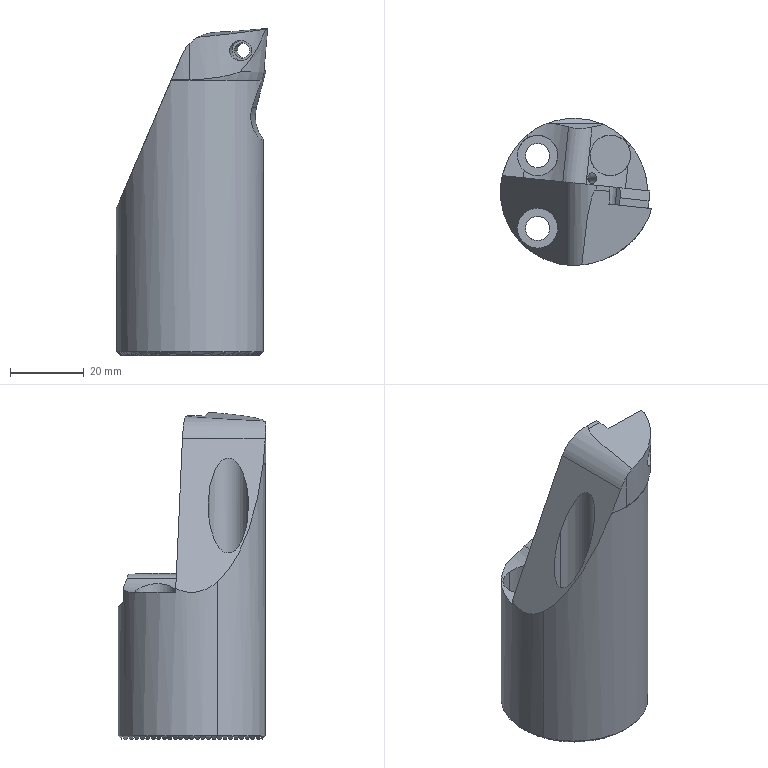Part | 2 solids | 224 faces | volume 63363 mm3 | plane 177 | cylinder 34 | cone 12 | torus 1 | commonest cylinder face diameters 11 x8 6.6 x6 2.9 x2 4.2 x2 5.5 x2 10.3 x2